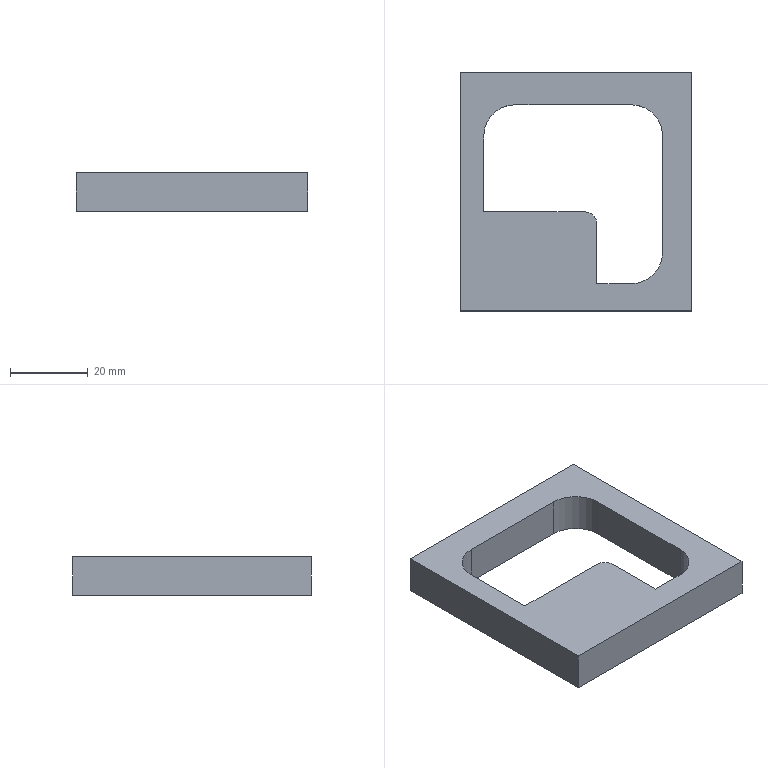Part | STEP file | Part 95^超升波生产线-2 | 1 solid | 16 faces | box 59.411 x 61.077 x 10 mm | volume 20947 mm3 | plane 12 | cylinder 4 | commonest cylinder face diameters 16 x3 6 x1
STEP:
#1=CARTESIAN_POINT('',(-23.115,144.153,0.));
#2=VERTEX_POINT('',#1);
#3=CARTESIAN_POINT('',(-23.115,83.076,0.));
#4=VERTEX_POINT('',#3);
#5=CARTESIAN_POINT('',(-23.115,144.153,0.));
#6=DIRECTION('',(0.,-1.,0.));
#7=VECTOR('',#6,1000.);
#8=LINE('',#5,#7);
#9=EDGE_CURVE('',#2,#4,#8,.T.);
#10=ORIENTED_EDGE('',*,*,#9,.T.);
#11=CARTESIAN_POINT('',(-23.115,83.076,10.));
#12=VERTEX_POINT('',#11);
#13=CARTESIAN_POINT('',(-23.115,83.076,10.));
#14=DIRECTION('',(0.,0.,-1.));
#15=VECTOR('',#14,1000.);
#16=LINE('',#13,#15);
#17=EDGE_CURVE('',#12,#4,#16,.T.);
#18=ORIENTED_EDGE('',*,*,#17,.F.);
#19=CARTESIAN_POINT('',(-23.115,144.153,10.));
#20=VERTEX_POINT('',#19);
#21=CARTESIAN_POINT('',(-23.115,144.153,10.));
#22=DIRECTION('',(0.,-1.,0.));
#23=VECTOR('',#22,1000.);
#24=LINE('',#21,#23);
#25=EDGE_CURVE('',#20,#12,#24,.T.);
#26=ORIENTED_EDGE('',*,*,#25,.F.);
#27=CARTESIAN_POINT('',(-23.115,144.153,10.));
#28=DIRECTION('',(0.,0.,-1.));
#29=VECTOR('',#28,1000.);
#30=LINE('',#27,#29);
#31=EDGE_CURVE('',#20,#2,#30,.T.);
#32=ORIENTED_EDGE('',*,*,#31,.T.);
#33=EDGE_LOOP('',(#10,#18,#26,#32));
#34=FACE_OUTER_BOUND('',#33,.T.);
#35=CARTESIAN_POINT('',(-23.115,144.153,10.));
#36=DIRECTION('',(1.,0.,0.));
#37=DIRECTION('',(0.,0.,-1.));
#38=AXIS2_PLACEMENT_3D('',#35,#36,#37);
#39=PLANE('',#38);
#40=ADVANCED_FACE('',(#34),#39,.F.);
#41=CARTESIAN_POINT('',(36.296,83.076,0.));
#42=VERTEX_POINT('',#41);
#43=CARTESIAN_POINT('',(-23.115,83.076,0.));
#44=DIRECTION('',(1.,0.,0.));
#45=VECTOR('',#44,1000.);
#46=LINE('',#43,#45);
#47=EDGE_CURVE('',#4,#42,#46,.T.);
#48=ORIENTED_EDGE('',*,*,#47,.T.);
#49=CARTESIAN_POINT('',(36.296,83.076,10.));
#50=VERTEX_POINT('',#49);
#51=CARTESIAN_POINT('',(36.296,83.076,10.));
#52=DIRECTION('',(0.,0.,-1.));
#53=VECTOR('',#52,1000.);
#54=LINE('',#51,#53);
#55=EDGE_CURVE('',#50,#42,#54,.T.);
#56=ORIENTED_EDGE('',*,*,#55,.F.);
#57=CARTESIAN_POINT('',(-23.115,83.076,10.));
#58=DIRECTION('',(1.,0.,0.));
#59=VECTOR('',#58,1000.);
#60=LINE('',#57,#59);
#61=EDGE_CURVE('',#12,#50,#60,.T.);
#62=ORIENTED_EDGE('',*,*,#61,.F.);
#63=ORIENTED_EDGE('',*,*,#17,.T.);
#64=EDGE_LOOP('',(#48,#56,#62,#63));
#65=FACE_OUTER_BOUND('',#64,.T.);
#66=CARTESIAN_POINT('',(-23.115,83.076,10.));
#67=DIRECTION('',(0.,1.,0.));
#68=DIRECTION('',(0.,0.,1.));
#69=AXIS2_PLACEMENT_3D('',#66,#67,#68);
#70=PLANE('',#69);
#71=ADVANCED_FACE('',(#65),#70,.F.);
#72=CARTESIAN_POINT('',(36.296,144.153,0.));
#73=VERTEX_POINT('',#72);
#74=CARTESIAN_POINT('',(36.296,144.153,0.));
#75=DIRECTION('',(0.,1.,0.));
#76=VECTOR('',#75,1000.);
#77=LINE('',#74,#76);
#78=EDGE_CURVE('',#42,#73,#77,.T.);
#79=ORIENTED_EDGE('',*,*,#78,.T.);
#80=CARTESIAN_POINT('',(36.296,144.153,10.));
#81=VERTEX_POINT('',#80);
#82=CARTESIAN_POINT('',(36.296,144.153,10.));
#83=DIRECTION('',(0.,0.,-1.));
#84=VECTOR('',#83,1000.);
#85=LINE('',#82,#84);
#86=EDGE_CURVE('',#81,#73,#85,.T.);
#87=ORIENTED_EDGE('',*,*,#86,.F.);
#88=CARTESIAN_POINT('',(36.296,144.153,10.));
#89=DIRECTION('',(0.,1.,0.));
#90=VECTOR('',#89,1000.);
#91=LINE('',#88,#90);
#92=EDGE_CURVE('',#50,#81,#91,.T.);
#93=ORIENTED_EDGE('',*,*,#92,.F.);
#94=ORIENTED_EDGE('',*,*,#55,.T.);
#95=EDGE_LOOP('',(#79,#87,#93,#94));
#96=FACE_OUTER_BOUND('',#95,.T.);
#97=CARTESIAN_POINT('',(36.296,144.153,10.));
#98=DIRECTION('',(-1.,0.,0.));
#99=DIRECTION('',(0.,0.,1.));
#100=AXIS2_PLACEMENT_3D('',#97,#98,#99);
#101=PLANE('',#100);
#102=ADVANCED_FACE('',(#96),#101,.F.);
#103=CARTESIAN_POINT('',(-23.115,144.153,0.));
#104=DIRECTION('',(-1.,0.,0.));
#105=VECTOR('',#104,1000.);
#106=LINE('',#103,#105);
#107=EDGE_CURVE('',#73,#2,#106,.T.);
#108=ORIENTED_EDGE('',*,*,#107,.T.);
#109=ORIENTED_EDGE('',*,*,#31,.F.);
#110=CARTESIAN_POINT('',(-23.115,144.153,10.));
#111=DIRECTION('',(-1.,0.,0.));
#112=VECTOR('',#111,1000.);
#113=LINE('',#110,#112);
#114=EDGE_CURVE('',#81,#20,#113,.T.);
#115=ORIENTED_EDGE('',*,*,#114,.F.);
#116=ORIENTED_EDGE('',*,*,#86,.T.);
#117=EDGE_LOOP('',(#108,#109,#115,#116));
#118=FACE_OUTER_BOUND('',#117,.T.);
#119=CARTESIAN_POINT('',(-23.115,144.153,10.));
#120=DIRECTION('',(0.,-1.,0.));
#121=DIRECTION('',(0.,0.,-1.));
#122=AXIS2_PLACEMENT_3D('',#119,#120,#121);
#123=PLANE('',#122);
#124=ADVANCED_FACE('',(#118),#123,.F.);
#125=CARTESIAN_POINT('',(11.922,105.484,10.));
#126=VERTEX_POINT('',#125);
#127=CARTESIAN_POINT('',(11.922,90.084,10.));
#128=VERTEX_POINT('',#127);
#129=CARTESIAN_POINT('',(11.922,90.084,10.));
#130=DIRECTION('',(0.,-1.,0.));
#131=VECTOR('',#130,1000.);
#132=LINE('',#129,#131);
#133=EDGE_CURVE('',#126,#128,#132,.T.);
#134=ORIENTED_EDGE('',*,*,#133,.F.);
#135=CARTESIAN_POINT('',(8.922,108.484,10.));
#136=VERTEX_POINT('',#135);
#137=CARTESIAN_POINT('',(8.922,105.484,10.));
#138=DIRECTION('',(0.,0.,-1.));
#139=DIRECTION('',(1.,0.,0.));
#140=AXIS2_PLACEMENT_3D('',#137,#138,#139);
#141=CIRCLE('',#140,3.);
#142=EDGE_CURVE('',#136,#126,#141,.T.);
#143=ORIENTED_EDGE('',*,*,#142,.F.);
#144=CARTESIAN_POINT('',(-17.078,108.484,10.));
#145=VERTEX_POINT('',#144);
#146=CARTESIAN_POINT('',(-17.078,108.484,10.));
#147=DIRECTION('',(1.,0.,0.));
#148=VECTOR('',#147,1000.);
#149=LINE('',#146,#148);
#150=EDGE_CURVE('',#145,#136,#149,.T.);
#151=ORIENTED_EDGE('',*,*,#150,.F.);
#152=CARTESIAN_POINT('',(-17.078,127.984,10.));
#153=VERTEX_POINT('',#152);
#154=CARTESIAN_POINT('',(-17.078,127.984,10.));
#155=DIRECTION('',(0.,-1.,0.));
#156=VECTOR('',#155,1000.);
#157=LINE('',#154,#156);
#158=EDGE_CURVE('',#153,#145,#157,.T.);
#159=ORIENTED_EDGE('',*,*,#158,.F.);
#160=CARTESIAN_POINT('',(-9.078,135.984,10.));
#161=VERTEX_POINT('',#160);
#162=CARTESIAN_POINT('',(-9.078,127.984,10.));
#163=DIRECTION('',(0.,0.,1.));
#164=DIRECTION('',(-1.,0.,0.));
#165=AXIS2_PLACEMENT_3D('',#162,#163,#164);
#166=CIRCLE('',#165,8.);
#167=EDGE_CURVE('',#161,#153,#166,.T.);
#168=ORIENTED_EDGE('',*,*,#167,.F.);
#169=CARTESIAN_POINT('',(20.822,135.984,10.));
#170=VERTEX_POINT('',#169);
#171=CARTESIAN_POINT('',(20.822,135.984,10.));
#172=DIRECTION('',(-1.,0.,0.));
#173=VECTOR('',#172,1000.);
#174=LINE('',#171,#173);
#175=EDGE_CURVE('',#170,#161,#174,.T.);
#176=ORIENTED_EDGE('',*,*,#175,.F.);
#177=CARTESIAN_POINT('',(28.822,127.984,10.));
#178=VERTEX_POINT('',#177);
#179=CARTESIAN_POINT('',(20.822,127.984,10.));
#180=DIRECTION('',(0.,0.,1.));
#181=DIRECTION('',(1.,0.,0.));
#182=AXIS2_PLACEMENT_3D('',#179,#180,#181);
#183=CIRCLE('',#182,8.);
#184=EDGE_CURVE('',#178,#170,#183,.T.);
#185=ORIENTED_EDGE('',*,*,#184,.F.);
#186=CARTESIAN_POINT('',(28.822,98.084,10.));
#187=VERTEX_POINT('',#186);
#188=CARTESIAN_POINT('',(28.822,98.084,10.));
#189=DIRECTION('',(0.,1.,0.));
#190=VECTOR('',#189,1000.);
#191=LINE('',#188,#190);
#192=EDGE_CURVE('',#187,#178,#191,.T.);
#193=ORIENTED_EDGE('',*,*,#192,.F.);
#194=CARTESIAN_POINT('',(20.822,90.084,10.));
#195=VERTEX_POINT('',#194);
#196=CARTESIAN_POINT('',(20.822,98.084,10.));
#197=DIRECTION('',(0.,0.,1.));
#198=DIRECTION('',(1.,0.,0.));
#199=AXIS2_PLACEMENT_3D('',#196,#197,#198);
#200=CIRCLE('',#199,8.);
#201=EDGE_CURVE('',#195,#187,#200,.T.);
#202=ORIENTED_EDGE('',*,*,#201,.F.);
#203=CARTESIAN_POINT('',(11.922,90.084,10.));
#204=DIRECTION('',(1.,0.,0.));
#205=VECTOR('',#204,1000.);
#206=LINE('',#203,#205);
#207=EDGE_CURVE('',#128,#195,#206,.T.);
#208=ORIENTED_EDGE('',*,*,#207,.F.);
#209=EDGE_LOOP('',(#134,#143,#151,#159,#168,#176,#185,#193,#202,#208));
#210=FACE_BOUND('',#209,.T.);
#211=ORIENTED_EDGE('',*,*,#25,.T.);
#212=ORIENTED_EDGE('',*,*,#61,.T.);
#213=ORIENTED_EDGE('',*,*,#92,.T.);
#214=ORIENTED_EDGE('',*,*,#114,.T.);
#215=EDGE_LOOP('',(#211,#212,#213,#214));
#216=FACE_OUTER_BOUND('',#215,.T.);
#217=CARTESIAN_POINT('',(-23.115,83.076,10.));
#218=DIRECTION('',(0.,0.,1.));
#219=DIRECTION('',(1.,0.,0.));
#220=AXIS2_PLACEMENT_3D('',#217,#218,#219);
#221=PLANE('',#220);
#222=ADVANCED_FACE('',(#210,#216),#221,.T.);
#223=CARTESIAN_POINT('',(8.922,108.484,0.));
#224=VERTEX_POINT('',#223);
#225=CARTESIAN_POINT('',(11.922,105.484,0.));
#226=VERTEX_POINT('',#225);
#227=CARTESIAN_POINT('',(8.922,105.484,0.));
#228=DIRECTION('',(0.,0.,-1.));
#229=DIRECTION('',(1.,0.,0.));
#230=AXIS2_PLACEMENT_3D('',#227,#228,#229);
#231=CIRCLE('',#230,3.);
#232=EDGE_CURVE('',#224,#226,#231,.T.);
#233=ORIENTED_EDGE('',*,*,#232,.T.);
#234=CARTESIAN_POINT('',(11.922,90.084,0.));
#235=VERTEX_POINT('',#234);
#236=CARTESIAN_POINT('',(11.922,90.084,0.));
#237=DIRECTION('',(0.,-1.,0.));
#238=VECTOR('',#237,1000.);
#239=LINE('',#236,#238);
#240=EDGE_CURVE('',#226,#235,#239,.T.);
#241=ORIENTED_EDGE('',*,*,#240,.T.);
#242=CARTESIAN_POINT('',(20.822,90.084,0.));
#243=VERTEX_POINT('',#242);
#244=CARTESIAN_POINT('',(11.922,90.084,0.));
#245=DIRECTION('',(1.,0.,0.));
#246=VECTOR('',#245,1000.);
#247=LINE('',#244,#246);
#248=EDGE_CURVE('',#235,#243,#247,.T.);
#249=ORIENTED_EDGE('',*,*,#248,.T.);
#250=CARTESIAN_POINT('',(28.822,98.084,0.));
#251=VERTEX_POINT('',#250);
#252=CARTESIAN_POINT('',(20.822,98.084,0.));
#253=DIRECTION('',(0.,0.,1.));
#254=DIRECTION('',(1.,0.,0.));
#255=AXIS2_PLACEMENT_3D('',#252,#253,#254);
#256=CIRCLE('',#255,8.);
#257=EDGE_CURVE('',#243,#251,#256,.T.);
#258=ORIENTED_EDGE('',*,*,#257,.T.);
#259=CARTESIAN_POINT('',(28.822,127.984,0.));
#260=VERTEX_POINT('',#259);
#261=CARTESIAN_POINT('',(28.822,98.084,0.));
#262=DIRECTION('',(0.,1.,0.));
#263=VECTOR('',#262,1000.);
#264=LINE('',#261,#263);
#265=EDGE_CURVE('',#251,#260,#264,.T.);
#266=ORIENTED_EDGE('',*,*,#265,.T.);
#267=CARTESIAN_POINT('',(20.822,135.984,0.));
#268=VERTEX_POINT('',#267);
#269=CARTESIAN_POINT('',(20.822,127.984,0.));
#270=DIRECTION('',(0.,0.,1.));
#271=DIRECTION('',(1.,0.,0.));
#272=AXIS2_PLACEMENT_3D('',#269,#270,#271);
#273=CIRCLE('',#272,8.);
#274=EDGE_CURVE('',#260,#268,#273,.T.);
#275=ORIENTED_EDGE('',*,*,#274,.T.);
#276=CARTESIAN_POINT('',(-9.078,135.984,0.));
#277=VERTEX_POINT('',#276);
#278=CARTESIAN_POINT('',(20.822,135.984,0.));
#279=DIRECTION('',(-1.,0.,0.));
#280=VECTOR('',#279,1000.);
#281=LINE('',#278,#280);
#282=EDGE_CURVE('',#268,#277,#281,.T.);
#283=ORIENTED_EDGE('',*,*,#282,.T.);
#284=CARTESIAN_POINT('',(-17.078,127.984,0.));
#285=VERTEX_POINT('',#284);
#286=CARTESIAN_POINT('',(-9.078,127.984,0.));
#287=DIRECTION('',(0.,0.,1.));
#288=DIRECTION('',(-1.,0.,0.));
#289=AXIS2_PLACEMENT_3D('',#286,#287,#288);
#290=CIRCLE('',#289,8.);
#291=EDGE_CURVE('',#277,#285,#290,.T.);
#292=ORIENTED_EDGE('',*,*,#291,.T.);
#293=CARTESIAN_POINT('',(-17.078,108.484,0.));
#294=VERTEX_POINT('',#293);
#295=CARTESIAN_POINT('',(-17.078,127.984,0.));
#296=DIRECTION('',(0.,-1.,0.));
#297=VECTOR('',#296,1000.);
#298=LINE('',#295,#297);
#299=EDGE_CURVE('',#285,#294,#298,.T.);
#300=ORIENTED_EDGE('',*,*,#299,.T.);
#301=CARTESIAN_POINT('',(-17.078,108.484,0.));
#302=DIRECTION('',(1.,0.,0.));
#303=VECTOR('',#302,1000.);
#304=LINE('',#301,#303);
#305=EDGE_CURVE('',#294,#224,#304,.T.);
#306=ORIENTED_EDGE('',*,*,#305,.T.);
#307=EDGE_LOOP('',(#233,#241,#249,#258,#266,#275,#283,#292,#300,#306));
#308=FACE_BOUND('',#307,.T.);
#309=ORIENTED_EDGE('',*,*,#9,.F.);
#310=ORIENTED_EDGE('',*,*,#107,.F.);
#311=ORIENTED_EDGE('',*,*,#78,.F.);
#312=ORIENTED_EDGE('',*,*,#47,.F.);
#313=EDGE_LOOP('',(#309,#310,#311,#312));
#314=FACE_OUTER_BOUND('',#313,.T.);
#315=CARTESIAN_POINT('',(-23.115,83.076,0.));
#316=DIRECTION('',(0.,0.,1.));
#317=DIRECTION('',(1.,0.,0.));
#318=AXIS2_PLACEMENT_3D('',#315,#316,#317);
#319=PLANE('',#318);
#320=ADVANCED_FACE('',(#308,#314),#319,.F.);
#321=ORIENTED_EDGE('',*,*,#133,.T.);
#322=CARTESIAN_POINT('',(11.922,90.084,0.));
#323=DIRECTION('',(0.,0.,1.));
#324=VECTOR('',#323,1000.);
#325=LINE('',#322,#324);
#326=EDGE_CURVE('',#235,#128,#325,.T.);
#327=ORIENTED_EDGE('',*,*,#326,.F.);
#328=ORIENTED_EDGE('',*,*,#240,.F.);
#329=CARTESIAN_POINT('',(11.922,105.484,0.));
#330=DIRECTION('',(0.,0.,1.));
#331=VECTOR('',#330,1000.);
#332=LINE('',#329,#331);
#333=EDGE_CURVE('',#226,#126,#332,.T.);
#334=ORIENTED_EDGE('',*,*,#333,.T.);
#335=EDGE_LOOP('',(#321,#327,#328,#334));
#336=FACE_OUTER_BOUND('',#335,.T.);
#337=CARTESIAN_POINT('',(11.922,90.084,0.));
#338=DIRECTION('',(-1.,0.,0.));
#339=DIRECTION('',(0.,0.,1.));
#340=AXIS2_PLACEMENT_3D('',#337,#338,#339);
#341=PLANE('',#340);
#342=ADVANCED_FACE('',(#336),#341,.F.);
#343=ORIENTED_EDGE('',*,*,#142,.T.);
#344=ORIENTED_EDGE('',*,*,#333,.F.);
#345=ORIENTED_EDGE('',*,*,#232,.F.);
#346=CARTESIAN_POINT('',(8.922,108.484,0.));
#347=DIRECTION('',(0.,0.,1.));
#348=VECTOR('',#347,1000.);
#349=LINE('',#346,#348);
#350=EDGE_CURVE('',#224,#136,#349,.T.);
#351=ORIENTED_EDGE('',*,*,#350,.T.);
#352=EDGE_LOOP('',(#343,#344,#345,#351));
#353=FACE_OUTER_BOUND('',#352,.T.);
#354=CARTESIAN_POINT('',(8.922,105.484,0.));
#355=DIRECTION('',(0.,0.,1.));
#356=DIRECTION('',(1.,0.,0.));
#357=AXIS2_PLACEMENT_3D('',#354,#355,#356);
#358=CYLINDRICAL_SURFACE('',#357,3.);
#359=ADVANCED_FACE('',(#353),#358,.T.);
#360=ORIENTED_EDGE('',*,*,#150,.T.);
#361=ORIENTED_EDGE('',*,*,#350,.F.);
#362=ORIENTED_EDGE('',*,*,#305,.F.);
#363=CARTESIAN_POINT('',(-17.078,108.484,0.));
#364=DIRECTION('',(0.,0.,1.));
#365=VECTOR('',#364,1000.);
#366=LINE('',#363,#365);
#367=EDGE_CURVE('',#294,#145,#366,.T.);
#368=ORIENTED_EDGE('',*,*,#367,.T.);
#369=EDGE_LOOP('',(#360,#361,#362,#368));
#370=FACE_OUTER_BOUND('',#369,.T.);
#371=CARTESIAN_POINT('',(-17.078,108.484,0.));
#372=DIRECTION('',(0.,-1.,0.));
#373=DIRECTION('',(0.,0.,-1.));
#374=AXIS2_PLACEMENT_3D('',#371,#372,#373);
#375=PLANE('',#374);
#376=ADVANCED_FACE('',(#370),#375,.F.);
#377=ORIENTED_EDGE('',*,*,#158,.T.);
#378=ORIENTED_EDGE('',*,*,#367,.F.);
#379=ORIENTED_EDGE('',*,*,#299,.F.);
#380=CARTESIAN_POINT('',(-17.078,127.984,0.));
#381=DIRECTION('',(0.,0.,1.));
#382=VECTOR('',#381,1000.);
#383=LINE('',#380,#382);
#384=EDGE_CURVE('',#285,#153,#383,.T.);
#385=ORIENTED_EDGE('',*,*,#384,.T.);
#386=EDGE_LOOP('',(#377,#378,#379,#385));
#387=FACE_OUTER_BOUND('',#386,.T.);
#388=CARTESIAN_POINT('',(-17.078,127.984,0.));
#389=DIRECTION('',(-1.,0.,0.));
#390=DIRECTION('',(0.,0.,1.));
#391=AXIS2_PLACEMENT_3D('',#388,#389,#390);
#392=PLANE('',#391);
#393=ADVANCED_FACE('',(#387),#392,.F.);
#394=ORIENTED_EDGE('',*,*,#167,.T.);
#395=ORIENTED_EDGE('',*,*,#384,.F.);
#396=ORIENTED_EDGE('',*,*,#291,.F.);
#397=CARTESIAN_POINT('',(-9.078,135.984,0.));
#398=DIRECTION('',(0.,0.,1.));
#399=VECTOR('',#398,1000.);
#400=LINE('',#397,#399);
#401=EDGE_CURVE('',#277,#161,#400,.T.);
#402=ORIENTED_EDGE('',*,*,#401,.T.);
#403=EDGE_LOOP('',(#394,#395,#396,#402));
#404=FACE_OUTER_BOUND('',#403,.T.);
#405=CARTESIAN_POINT('',(-9.078,127.984,0.));
#406=DIRECTION('',(0.,0.,1.));
#407=DIRECTION('',(1.,0.,0.));
#408=AXIS2_PLACEMENT_3D('',#405,#406,#407);
#409=CYLINDRICAL_SURFACE('',#408,8.);
#410=ADVANCED_FACE('',(#404),#409,.F.);
#411=ORIENTED_EDGE('',*,*,#175,.T.);
#412=ORIENTED_EDGE('',*,*,#401,.F.);
#413=ORIENTED_EDGE('',*,*,#282,.F.);
#414=CARTESIAN_POINT('',(20.822,135.984,0.));
#415=DIRECTION('',(0.,0.,1.));
#416=VECTOR('',#415,1000.);
#417=LINE('',#414,#416);
#418=EDGE_CURVE('',#268,#170,#417,.T.);
#419=ORIENTED_EDGE('',*,*,#418,.T.);
#420=EDGE_LOOP('',(#411,#412,#413,#419));
#421=FACE_OUTER_BOUND('',#420,.T.);
#422=CARTESIAN_POINT('',(20.822,135.984,0.));
#423=DIRECTION('',(0.,1.,0.));
#424=DIRECTION('',(0.,0.,1.));
#425=AXIS2_PLACEMENT_3D('',#422,#423,#424);
#426=PLANE('',#425);
#427=ADVANCED_FACE('',(#421),#426,.F.);
#428=ORIENTED_EDGE('',*,*,#184,.T.);
#429=ORIENTED_EDGE('',*,*,#418,.F.);
#430=ORIENTED_EDGE('',*,*,#274,.F.);
#431=CARTESIAN_POINT('',(28.822,127.984,0.));
#432=DIRECTION('',(0.,0.,1.));
#433=VECTOR('',#432,1000.);
#434=LINE('',#431,#433);
#435=EDGE_CURVE('',#260,#178,#434,.T.);
#436=ORIENTED_EDGE('',*,*,#435,.T.);
#437=EDGE_LOOP('',(#428,#429,#430,#436));
#438=FACE_OUTER_BOUND('',#437,.T.);
#439=CARTESIAN_POINT('',(20.822,127.984,0.));
#440=DIRECTION('',(0.,0.,1.));
#441=DIRECTION('',(1.,0.,0.));
#442=AXIS2_PLACEMENT_3D('',#439,#440,#441);
#443=CYLINDRICAL_SURFACE('',#442,8.);
#444=ADVANCED_FACE('',(#438),#443,.F.);
#445=ORIENTED_EDGE('',*,*,#192,.T.);
#446=ORIENTED_EDGE('',*,*,#435,.F.);
#447=ORIENTED_EDGE('',*,*,#265,.F.);
#448=CARTESIAN_POINT('',(28.822,98.084,0.));
#449=DIRECTION('',(0.,0.,1.));
#450=VECTOR('',#449,1000.);
#451=LINE('',#448,#450);
#452=EDGE_CURVE('',#251,#187,#451,.T.);
#453=ORIENTED_EDGE('',*,*,#452,.T.);
#454=EDGE_LOOP('',(#445,#446,#447,#453));
#455=FACE_OUTER_BOUND('',#454,.T.);
#456=CARTESIAN_POINT('',(28.822,98.084,0.));
#457=DIRECTION('',(1.,0.,0.));
#458=DIRECTION('',(0.,0.,-1.));
#459=AXIS2_PLACEMENT_3D('',#456,#457,#458);
#460=PLANE('',#459);
#461=ADVANCED_FACE('',(#455),#460,.F.);
#462=ORIENTED_EDGE('',*,*,#201,.T.);
#463=ORIENTED_EDGE('',*,*,#452,.F.);
#464=ORIENTED_EDGE('',*,*,#257,.F.);
#465=CARTESIAN_POINT('',(20.822,90.084,0.));
#466=DIRECTION('',(0.,0.,1.));
#467=VECTOR('',#466,1000.);
#468=LINE('',#465,#467);
#469=EDGE_CURVE('',#243,#195,#468,.T.);
#470=ORIENTED_EDGE('',*,*,#469,.T.);
#471=EDGE_LOOP('',(#462,#463,#464,#470));
#472=FACE_OUTER_BOUND('',#471,.T.);
#473=CARTESIAN_POINT('',(20.822,98.084,0.));
#474=DIRECTION('',(0.,0.,1.));
#475=DIRECTION('',(1.,0.,0.));
#476=AXIS2_PLACEMENT_3D('',#473,#474,#475);
#477=CYLINDRICAL_SURFACE('',#476,8.);
#478=ADVANCED_FACE('',(#472),#477,.F.);
#479=ORIENTED_EDGE('',*,*,#207,.T.);
#480=ORIENTED_EDGE('',*,*,#469,.F.);
#481=ORIENTED_EDGE('',*,*,#248,.F.);
#482=ORIENTED_EDGE('',*,*,#326,.T.);
#483=EDGE_LOOP('',(#479,#480,#481,#482));
#484=FACE_OUTER_BOUND('',#483,.T.);
#485=CARTESIAN_POINT('',(11.922,90.084,0.));
#486=DIRECTION('',(0.,-1.,0.));
#487=DIRECTION('',(0.,0.,-1.));
#488=AXIS2_PLACEMENT_3D('',#485,#486,#487);
#489=PLANE('',#488);
#490=ADVANCED_FACE('',(#484),#489,.F.);
#491=CLOSED_SHELL('',(#40,#71,#102,#124,#222,#320,#342,#359,#376,#393,#410,#427,#444,#461,#478,#490));
#492=MANIFOLD_SOLID_BREP('',#491);
#493=CARTESIAN_POINT('',(0.,0.,0.));
#494=DIRECTION('',(0.,0.,1.));
#495=DIRECTION('',(1.,0.,0.));
#496=AXIS2_PLACEMENT_3D('',#493,#494,#495);
#497=(LENGTH_UNIT()NAMED_UNIT(*)SI_UNIT(.MILLI.,.METRE.));
#498=UNCERTAINTY_MEASURE_WITH_UNIT(LENGTH_MEASURE(0.00001),#497,'','');
#499=(NAMED_UNIT(*)PLANE_ANGLE_UNIT()SI_UNIT($,.RADIAN.));
#500=(NAMED_UNIT(*)SI_UNIT($,.STERADIAN.)SOLID_ANGLE_UNIT());
#501=(GEOMETRIC_REPRESENTATION_CONTEXT(3)GLOBAL_UNCERTAINTY_ASSIGNED_CONTEXT((#498))GLOBAL_UNIT_ASSIGNED_CONTEXT((#497,#499,#500))REPRESENTATION_CONTEXT('',''));
#502=ADVANCED_BREP_SHAPE_REPRESENTATION('',(#492,#496),#501);